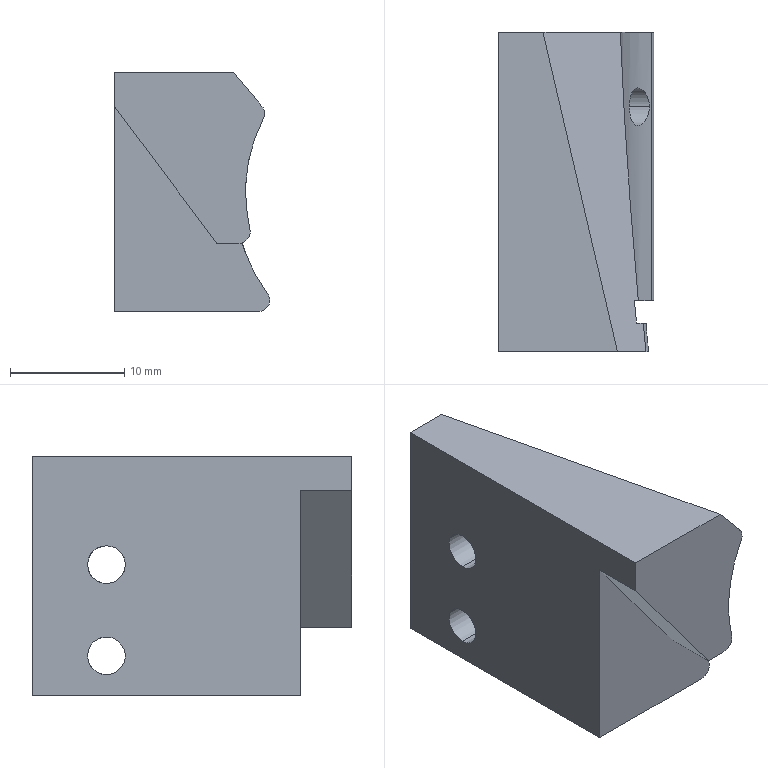Part | STEP file | CLM-5001A | 1 solid | 20 faces | box 13.626 x 28 x 21 mm | volume 5621 mm3 | plane 10 | cylinder 9 | spline 1 | commonest cylinder face diameters 3.3 x4 2 x2 28 x1 30 x1 31 x1